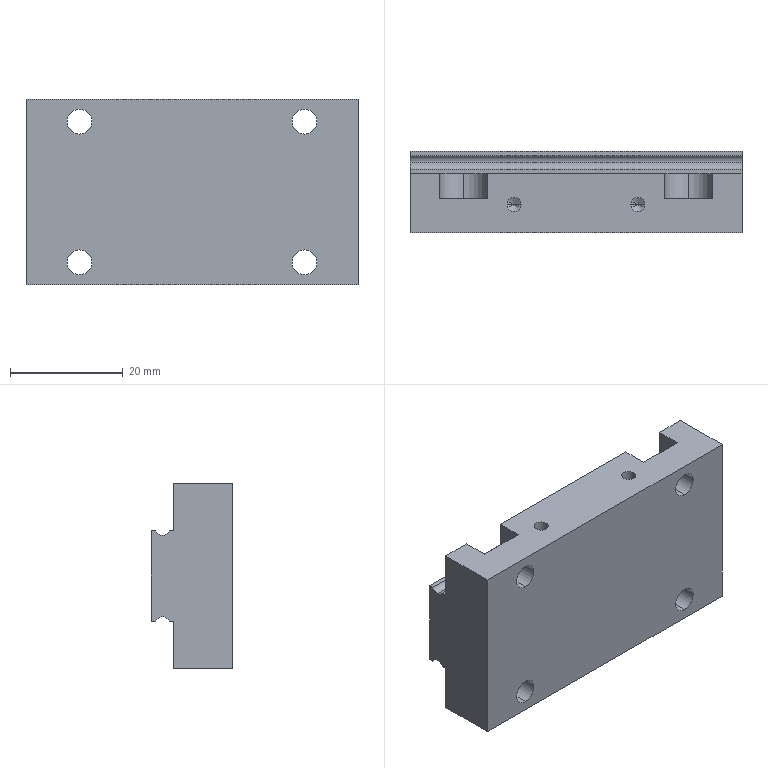Part | NX | 1 solid | 57 faces | box 59 x 14.5 x 33 mm | volume 22446 mm3 | cylinder 25 | plane 24 | cone 8 | commonest cylinder face diameters 2.5 x8 4.4 x8 8.5 x6 2.7 x3